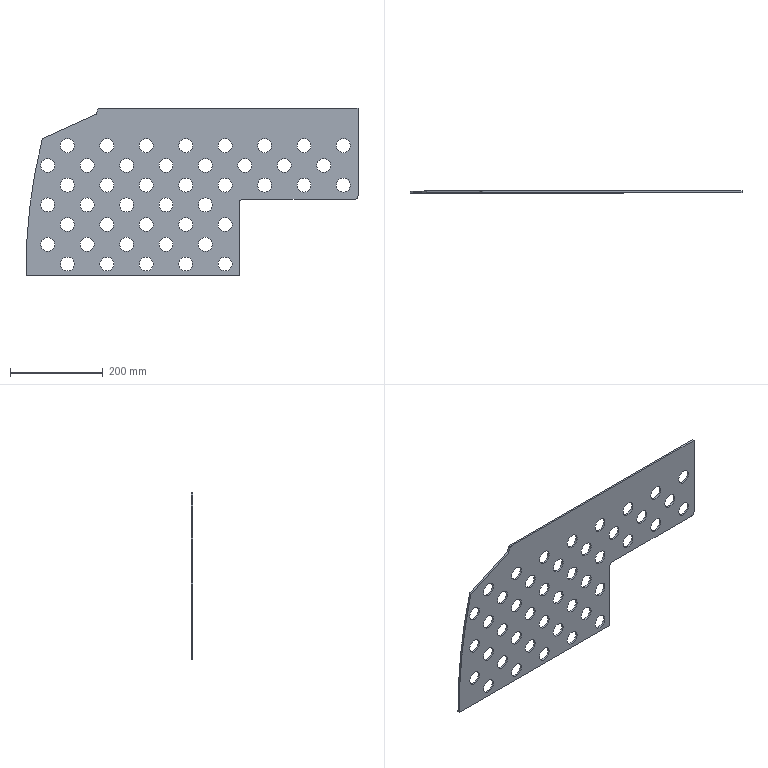Part | SolidWorks | features Extrusion 1 | 1 solid | 103 faces | box 714.557 x 4 x 360 mm | volume 695889 mm3 | cylinder 94 | plane 9 | commonest cylinder face diameters 30 x88 10 x3 16 x2 2302 x1